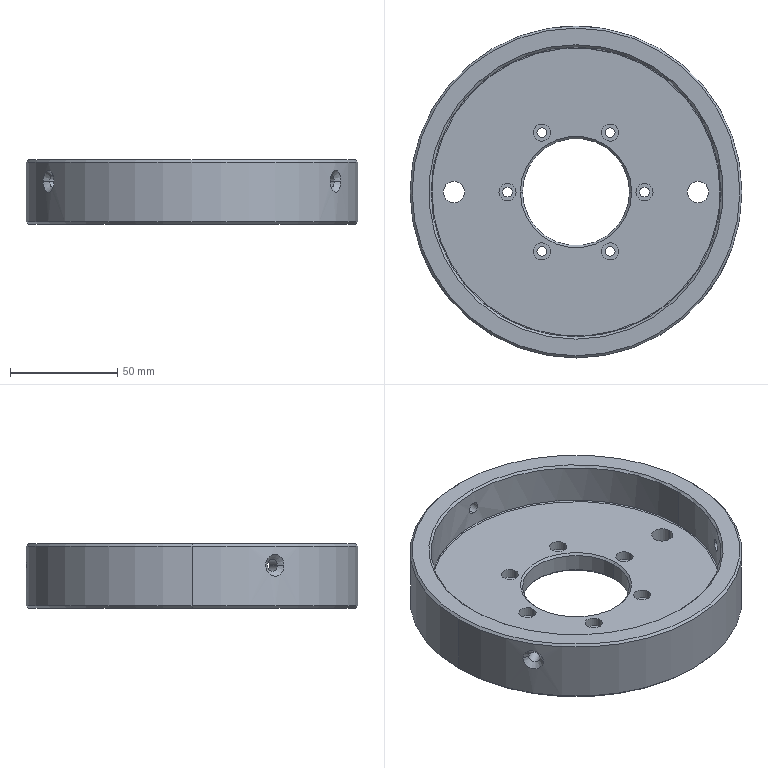Part | STEP file | Hub mounting plate | 1 solid | 67 faces | box 155 x 155 x 30 mm | volume 252907 mm3 | cylinder 40 | cone 16 | plane 9 | spline 2 | commonest cylinder face diameters 4.5 x12 8 x12 5.5 x6 10 x4 50 x2 135.5 x2